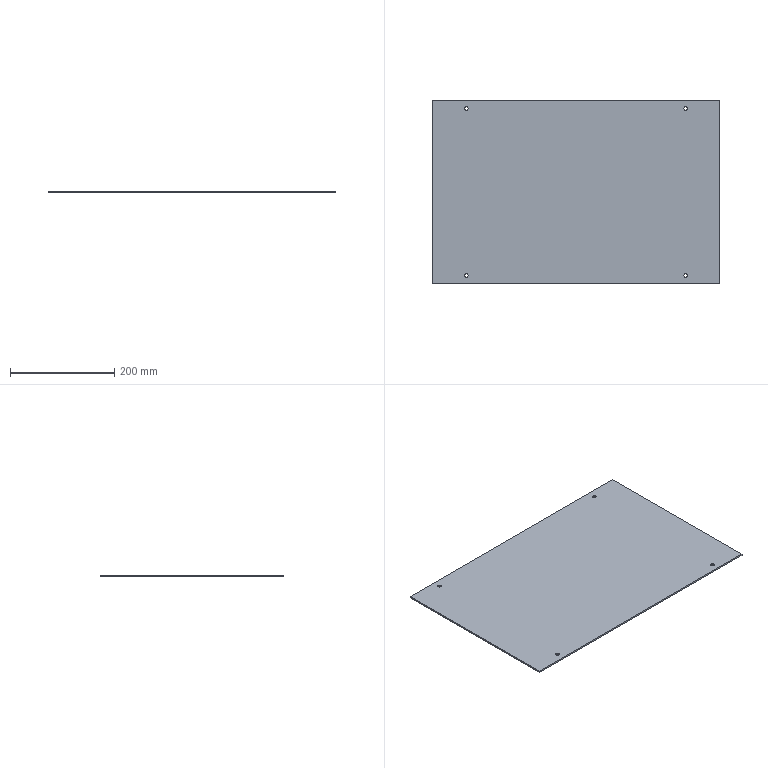Part | SolidWorks | features BaseBody 1 | 1 solid | 14 faces | box 550 x 350 x 3 mm | volume 577089 mm3 | cylinder 8 | plane 6 | commonest cylinder face diameters 6.6 x8
STEP:
#1=CARTESIAN_POINT('',(206.7,160.,0.));
#2=VERTEX_POINT('',#1);
#3=CARTESIAN_POINT('',(213.3,160.,0.));
#4=VERTEX_POINT('',#3);
#5=CARTESIAN_POINT('',(210.,160.,0.));
#6=DIRECTION('',(0.,0.,1.));
#7=DIRECTION('',(-1.,0.,0.));
#8=AXIS2_PLACEMENT_3D('',#5,#6,#7);
#9=CIRCLE('',#8,3.3);
#10=EDGE_CURVE('',#2,#4,#9,.T.);
#11=ORIENTED_EDGE('',*,*,#10,.T.);
#12=CARTESIAN_POINT('',(213.3,160.,-3.));
#13=VERTEX_POINT('',#12);
#14=CARTESIAN_POINT('',(213.3,160.,0.));
#15=DIRECTION('',(0.,0.,-1.));
#16=VECTOR('',#15,1000.);
#17=LINE('',#14,#16);
#18=EDGE_CURVE('',#4,#13,#17,.T.);
#19=ORIENTED_EDGE('',*,*,#18,.T.);
#20=CARTESIAN_POINT('',(206.7,160.,-3.));
#21=VERTEX_POINT('',#20);
#22=CARTESIAN_POINT('',(210.,160.,-3.));
#23=DIRECTION('',(0.,0.,-1.));
#24=DIRECTION('',(-1.,0.,0.));
#25=AXIS2_PLACEMENT_3D('',#22,#23,#24);
#26=CIRCLE('',#25,3.3);
#27=EDGE_CURVE('',#13,#21,#26,.T.);
#28=ORIENTED_EDGE('',*,*,#27,.T.);
#29=CARTESIAN_POINT('',(206.7,160.,0.));
#30=DIRECTION('',(0.,0.,-1.));
#31=VECTOR('',#30,1000.);
#32=LINE('',#29,#31);
#33=EDGE_CURVE('',#2,#21,#32,.T.);
#34=ORIENTED_EDGE('',*,*,#33,.F.);
#35=EDGE_LOOP('',(#11,#19,#28,#34));
#36=FACE_OUTER_BOUND('',#35,.T.);
#37=CARTESIAN_POINT('',(210.,160.,0.));
#38=DIRECTION('',(0.,0.,-1.));
#39=DIRECTION('',(-1.,0.,0.));
#40=AXIS2_PLACEMENT_3D('',#37,#38,#39);
#41=CYLINDRICAL_SURFACE('',#40,3.3);
#42=ADVANCED_FACE('',(#36),#41,.F.);
#43=CARTESIAN_POINT('',(-213.3,160.,0.));
#44=VERTEX_POINT('',#43);
#45=CARTESIAN_POINT('',(-206.7,160.,0.));
#46=VERTEX_POINT('',#45);
#47=CARTESIAN_POINT('',(-210.,160.,0.));
#48=DIRECTION('',(0.,0.,1.));
#49=DIRECTION('',(-1.,0.,0.));
#50=AXIS2_PLACEMENT_3D('',#47,#48,#49);
#51=CIRCLE('',#50,3.3);
#52=EDGE_CURVE('',#44,#46,#51,.T.);
#53=ORIENTED_EDGE('',*,*,#52,.T.);
#54=CARTESIAN_POINT('',(-206.7,160.,-3.));
#55=VERTEX_POINT('',#54);
#56=CARTESIAN_POINT('',(-206.7,160.,0.));
#57=DIRECTION('',(0.,0.,-1.));
#58=VECTOR('',#57,1000.);
#59=LINE('',#56,#58);
#60=EDGE_CURVE('',#46,#55,#59,.T.);
#61=ORIENTED_EDGE('',*,*,#60,.T.);
#62=CARTESIAN_POINT('',(-213.3,160.,-3.));
#63=VERTEX_POINT('',#62);
#64=CARTESIAN_POINT('',(-210.,160.,-3.));
#65=DIRECTION('',(0.,0.,1.));
#66=DIRECTION('',(-1.,0.,0.));
#67=AXIS2_PLACEMENT_3D('',#64,#65,#66);
#68=CIRCLE('',#67,3.3);
#69=EDGE_CURVE('',#63,#55,#68,.T.);
#70=ORIENTED_EDGE('',*,*,#69,.F.);
#71=CARTESIAN_POINT('',(-213.3,160.,0.));
#72=DIRECTION('',(0.,0.,-1.));
#73=VECTOR('',#72,1000.);
#74=LINE('',#71,#73);
#75=EDGE_CURVE('',#44,#63,#74,.T.);
#76=ORIENTED_EDGE('',*,*,#75,.F.);
#77=EDGE_LOOP('',(#53,#61,#70,#76));
#78=FACE_OUTER_BOUND('',#77,.T.);
#79=CARTESIAN_POINT('',(-210.,160.,0.));
#80=DIRECTION('',(0.,0.,-1.));
#81=DIRECTION('',(-1.,0.,0.));
#82=AXIS2_PLACEMENT_3D('',#79,#80,#81);
#83=CYLINDRICAL_SURFACE('',#82,3.3);
#84=ADVANCED_FACE('',(#78),#83,.F.);
#85=CARTESIAN_POINT('',(-213.3,-160.,0.));
#86=VERTEX_POINT('',#85);
#87=CARTESIAN_POINT('',(-206.7,-160.,0.));
#88=VERTEX_POINT('',#87);
#89=CARTESIAN_POINT('',(-210.,-160.,0.));
#90=DIRECTION('',(0.,0.,1.));
#91=DIRECTION('',(-1.,0.,0.));
#92=AXIS2_PLACEMENT_3D('',#89,#90,#91);
#93=CIRCLE('',#92,3.3);
#94=EDGE_CURVE('',#86,#88,#93,.T.);
#95=ORIENTED_EDGE('',*,*,#94,.T.);
#96=CARTESIAN_POINT('',(-206.7,-160.,-3.));
#97=VERTEX_POINT('',#96);
#98=CARTESIAN_POINT('',(-206.7,-160.,0.));
#99=DIRECTION('',(0.,0.,-1.));
#100=VECTOR('',#99,1000.);
#101=LINE('',#98,#100);
#102=EDGE_CURVE('',#88,#97,#101,.T.);
#103=ORIENTED_EDGE('',*,*,#102,.T.);
#104=CARTESIAN_POINT('',(-213.3,-160.,-3.));
#105=VERTEX_POINT('',#104);
#106=CARTESIAN_POINT('',(-210.,-160.,-3.));
#107=DIRECTION('',(0.,0.,1.));
#108=DIRECTION('',(-1.,0.,0.));
#109=AXIS2_PLACEMENT_3D('',#106,#107,#108);
#110=CIRCLE('',#109,3.3);
#111=EDGE_CURVE('',#105,#97,#110,.T.);
#112=ORIENTED_EDGE('',*,*,#111,.F.);
#113=CARTESIAN_POINT('',(-213.3,-160.,0.));
#114=DIRECTION('',(0.,0.,-1.));
#115=VECTOR('',#114,1000.);
#116=LINE('',#113,#115);
#117=EDGE_CURVE('',#86,#105,#116,.T.);
#118=ORIENTED_EDGE('',*,*,#117,.F.);
#119=EDGE_LOOP('',(#95,#103,#112,#118));
#120=FACE_OUTER_BOUND('',#119,.T.);
#121=CARTESIAN_POINT('',(-210.,-160.,0.));
#122=DIRECTION('',(0.,0.,-1.));
#123=DIRECTION('',(-1.,0.,0.));
#124=AXIS2_PLACEMENT_3D('',#121,#122,#123);
#125=CYLINDRICAL_SURFACE('',#124,3.3);
#126=ADVANCED_FACE('',(#120),#125,.F.);
#127=CARTESIAN_POINT('',(206.7,-160.,0.));
#128=VERTEX_POINT('',#127);
#129=CARTESIAN_POINT('',(213.3,-160.,0.));
#130=VERTEX_POINT('',#129);
#131=CARTESIAN_POINT('',(210.,-160.,0.));
#132=DIRECTION('',(0.,0.,1.));
#133=DIRECTION('',(-1.,0.,0.));
#134=AXIS2_PLACEMENT_3D('',#131,#132,#133);
#135=CIRCLE('',#134,3.3);
#136=EDGE_CURVE('',#128,#130,#135,.T.);
#137=ORIENTED_EDGE('',*,*,#136,.T.);
#138=CARTESIAN_POINT('',(213.3,-160.,-3.));
#139=VERTEX_POINT('',#138);
#140=CARTESIAN_POINT('',(213.3,-160.,0.));
#141=DIRECTION('',(0.,0.,-1.));
#142=VECTOR('',#141,1000.);
#143=LINE('',#140,#142);
#144=EDGE_CURVE('',#130,#139,#143,.T.);
#145=ORIENTED_EDGE('',*,*,#144,.T.);
#146=CARTESIAN_POINT('',(206.7,-160.,-3.));
#147=VERTEX_POINT('',#146);
#148=CARTESIAN_POINT('',(210.,-160.,-3.));
#149=DIRECTION('',(0.,0.,1.));
#150=DIRECTION('',(-1.,0.,0.));
#151=AXIS2_PLACEMENT_3D('',#148,#149,#150);
#152=CIRCLE('',#151,3.3);
#153=EDGE_CURVE('',#147,#139,#152,.T.);
#154=ORIENTED_EDGE('',*,*,#153,.F.);
#155=CARTESIAN_POINT('',(206.7,-160.,0.));
#156=DIRECTION('',(0.,0.,-1.));
#157=VECTOR('',#156,1000.);
#158=LINE('',#155,#157);
#159=EDGE_CURVE('',#128,#147,#158,.T.);
#160=ORIENTED_EDGE('',*,*,#159,.F.);
#161=EDGE_LOOP('',(#137,#145,#154,#160));
#162=FACE_OUTER_BOUND('',#161,.T.);
#163=CARTESIAN_POINT('',(210.,-160.,0.));
#164=DIRECTION('',(0.,0.,-1.));
#165=DIRECTION('',(-1.,0.,0.));
#166=AXIS2_PLACEMENT_3D('',#163,#164,#165);
#167=CYLINDRICAL_SURFACE('',#166,3.3);
#168=ADVANCED_FACE('',(#162),#167,.F.);
#169=ORIENTED_EDGE('',*,*,#18,.F.);
#170=CARTESIAN_POINT('',(210.,160.,0.));
#171=DIRECTION('',(0.,0.,1.));
#172=DIRECTION('',(-1.,0.,0.));
#173=AXIS2_PLACEMENT_3D('',#170,#171,#172);
#174=CIRCLE('',#173,3.3);
#175=EDGE_CURVE('',#4,#2,#174,.T.);
#176=ORIENTED_EDGE('',*,*,#175,.T.);
#177=ORIENTED_EDGE('',*,*,#33,.T.);
#178=CARTESIAN_POINT('',(210.,160.,-3.));
#179=DIRECTION('',(0.,0.,-1.));
#180=DIRECTION('',(-1.,0.,0.));
#181=AXIS2_PLACEMENT_3D('',#178,#179,#180);
#182=CIRCLE('',#181,3.3);
#183=EDGE_CURVE('',#21,#13,#182,.T.);
#184=ORIENTED_EDGE('',*,*,#183,.T.);
#185=EDGE_LOOP('',(#169,#176,#177,#184));
#186=FACE_OUTER_BOUND('',#185,.T.);
#187=CARTESIAN_POINT('',(210.,160.,0.));
#188=DIRECTION('',(0.,0.,-1.));
#189=DIRECTION('',(-1.,0.,0.));
#190=AXIS2_PLACEMENT_3D('',#187,#188,#189);
#191=CYLINDRICAL_SURFACE('',#190,3.3);
#192=ADVANCED_FACE('',(#186),#191,.F.);
#193=ORIENTED_EDGE('',*,*,#69,.T.);
#194=CARTESIAN_POINT('',(-210.,160.,-3.));
#195=DIRECTION('',(0.,0.,1.));
#196=DIRECTION('',(-1.,0.,0.));
#197=AXIS2_PLACEMENT_3D('',#194,#195,#196);
#198=CIRCLE('',#197,3.3);
#199=EDGE_CURVE('',#55,#63,#198,.T.);
#200=ORIENTED_EDGE('',*,*,#199,.T.);
#201=EDGE_LOOP('',(#193,#200));
#202=FACE_BOUND('',#201,.T.);
#203=ORIENTED_EDGE('',*,*,#111,.T.);
#204=CARTESIAN_POINT('',(-210.,-160.,-3.));
#205=DIRECTION('',(0.,0.,1.));
#206=DIRECTION('',(-1.,0.,0.));
#207=AXIS2_PLACEMENT_3D('',#204,#205,#206);
#208=CIRCLE('',#207,3.3);
#209=EDGE_CURVE('',#97,#105,#208,.T.);
#210=ORIENTED_EDGE('',*,*,#209,.T.);
#211=EDGE_LOOP('',(#203,#210));
#212=FACE_BOUND('',#211,.T.);
#213=ORIENTED_EDGE('',*,*,#153,.T.);
#214=CARTESIAN_POINT('',(210.,-160.,-3.));
#215=DIRECTION('',(0.,0.,1.));
#216=DIRECTION('',(-1.,0.,0.));
#217=AXIS2_PLACEMENT_3D('',#214,#215,#216);
#218=CIRCLE('',#217,3.3);
#219=EDGE_CURVE('',#139,#147,#218,.T.);
#220=ORIENTED_EDGE('',*,*,#219,.T.);
#221=EDGE_LOOP('',(#213,#220));
#222=FACE_BOUND('',#221,.T.);
#223=ORIENTED_EDGE('',*,*,#183,.F.);
#224=ORIENTED_EDGE('',*,*,#27,.F.);
#225=EDGE_LOOP('',(#223,#224));
#226=FACE_BOUND('',#225,.T.);
#227=CARTESIAN_POINT('',(-275.,-175.,-3.));
#228=VERTEX_POINT('',#227);
#229=CARTESIAN_POINT('',(-275.,175.,-3.));
#230=VERTEX_POINT('',#229);
#231=CARTESIAN_POINT('',(-275.,0.,-3.));
#232=DIRECTION('',(0.,1.,0.));
#233=VECTOR('',#232,1000.);
#234=LINE('',#231,#233);
#235=EDGE_CURVE('',#228,#230,#234,.T.);
#236=ORIENTED_EDGE('',*,*,#235,.T.);
#237=CARTESIAN_POINT('',(275.,175.,-3.));
#238=VERTEX_POINT('',#237);
#239=CARTESIAN_POINT('',(0.,175.,-3.));
#240=DIRECTION('',(1.,0.,0.));
#241=VECTOR('',#240,1000.);
#242=LINE('',#239,#241);
#243=EDGE_CURVE('',#230,#238,#242,.T.);
#244=ORIENTED_EDGE('',*,*,#243,.T.);
#245=CARTESIAN_POINT('',(275.,-175.,-3.));
#246=VERTEX_POINT('',#245);
#247=CARTESIAN_POINT('',(275.,0.,-3.));
#248=DIRECTION('',(0.,-1.,0.));
#249=VECTOR('',#248,1000.);
#250=LINE('',#247,#249);
#251=EDGE_CURVE('',#238,#246,#250,.T.);
#252=ORIENTED_EDGE('',*,*,#251,.T.);
#253=CARTESIAN_POINT('',(0.,-175.,-3.));
#254=DIRECTION('',(-1.,0.,0.));
#255=VECTOR('',#254,1000.);
#256=LINE('',#253,#255);
#257=EDGE_CURVE('',#246,#228,#256,.T.);
#258=ORIENTED_EDGE('',*,*,#257,.T.);
#259=EDGE_LOOP('',(#236,#244,#252,#258));
#260=FACE_OUTER_BOUND('',#259,.T.);
#261=CARTESIAN_POINT('',(275.,-175.,-3.));
#262=DIRECTION('',(0.,0.,-1.));
#263=DIRECTION('',(-1.,0.,0.));
#264=AXIS2_PLACEMENT_3D('',#261,#262,#263);
#265=PLANE('',#264);
#266=ADVANCED_FACE('',(#202,#212,#222,#226,#260),#265,.T.);
#267=ORIENTED_EDGE('',*,*,#52,.F.);
#268=CARTESIAN_POINT('',(-210.,160.,0.));
#269=DIRECTION('',(0.,0.,1.));
#270=DIRECTION('',(-1.,0.,0.));
#271=AXIS2_PLACEMENT_3D('',#268,#269,#270);
#272=CIRCLE('',#271,3.3);
#273=EDGE_CURVE('',#46,#44,#272,.T.);
#274=ORIENTED_EDGE('',*,*,#273,.F.);
#275=EDGE_LOOP('',(#267,#274));
#276=FACE_BOUND('',#275,.T.);
#277=ORIENTED_EDGE('',*,*,#94,.F.);
#278=CARTESIAN_POINT('',(-210.,-160.,0.));
#279=DIRECTION('',(0.,0.,1.));
#280=DIRECTION('',(-1.,0.,0.));
#281=AXIS2_PLACEMENT_3D('',#278,#279,#280);
#282=CIRCLE('',#281,3.3);
#283=EDGE_CURVE('',#88,#86,#282,.T.);
#284=ORIENTED_EDGE('',*,*,#283,.F.);
#285=EDGE_LOOP('',(#277,#284));
#286=FACE_BOUND('',#285,.T.);
#287=ORIENTED_EDGE('',*,*,#136,.F.);
#288=CARTESIAN_POINT('',(210.,-160.,0.));
#289=DIRECTION('',(0.,0.,1.));
#290=DIRECTION('',(-1.,0.,0.));
#291=AXIS2_PLACEMENT_3D('',#288,#289,#290);
#292=CIRCLE('',#291,3.3);
#293=EDGE_CURVE('',#130,#128,#292,.T.);
#294=ORIENTED_EDGE('',*,*,#293,.F.);
#295=EDGE_LOOP('',(#287,#294));
#296=FACE_BOUND('',#295,.T.);
#297=ORIENTED_EDGE('',*,*,#10,.F.);
#298=ORIENTED_EDGE('',*,*,#175,.F.);
#299=EDGE_LOOP('',(#297,#298));
#300=FACE_BOUND('',#299,.T.);
#301=CARTESIAN_POINT('',(-275.,175.,0.));
#302=VERTEX_POINT('',#301);
#303=CARTESIAN_POINT('',(275.,175.,0.));
#304=VERTEX_POINT('',#303);
#305=CARTESIAN_POINT('',(0.,175.,0.));
#306=DIRECTION('',(1.,0.,0.));
#307=VECTOR('',#306,1000.);
#308=LINE('',#305,#307);
#309=EDGE_CURVE('',#302,#304,#308,.T.);
#310=ORIENTED_EDGE('',*,*,#309,.F.);
#311=CARTESIAN_POINT('',(-275.,-175.,0.));
#312=VERTEX_POINT('',#311);
#313=CARTESIAN_POINT('',(-275.,0.,0.));
#314=DIRECTION('',(0.,1.,0.));
#315=VECTOR('',#314,1000.);
#316=LINE('',#313,#315);
#317=EDGE_CURVE('',#312,#302,#316,.T.);
#318=ORIENTED_EDGE('',*,*,#317,.F.);
#319=CARTESIAN_POINT('',(275.,-175.,0.));
#320=VERTEX_POINT('',#319);
#321=CARTESIAN_POINT('',(0.,-175.,0.));
#322=DIRECTION('',(-1.,0.,0.));
#323=VECTOR('',#322,1000.);
#324=LINE('',#321,#323);
#325=EDGE_CURVE('',#320,#312,#324,.T.);
#326=ORIENTED_EDGE('',*,*,#325,.F.);
#327=CARTESIAN_POINT('',(275.,0.,0.));
#328=DIRECTION('',(0.,-1.,0.));
#329=VECTOR('',#328,1000.);
#330=LINE('',#327,#329);
#331=EDGE_CURVE('',#304,#320,#330,.T.);
#332=ORIENTED_EDGE('',*,*,#331,.F.);
#333=EDGE_LOOP('',(#310,#318,#326,#332));
#334=FACE_OUTER_BOUND('',#333,.T.);
#335=CARTESIAN_POINT('',(275.,-175.,0.));
#336=DIRECTION('',(0.,0.,-1.));
#337=DIRECTION('',(-1.,0.,0.));
#338=AXIS2_PLACEMENT_3D('',#335,#336,#337);
#339=PLANE('',#338);
#340=ADVANCED_FACE('',(#276,#286,#296,#300,#334),#339,.F.);
#341=ORIENTED_EDGE('',*,*,#60,.F.);
#342=ORIENTED_EDGE('',*,*,#273,.T.);
#343=ORIENTED_EDGE('',*,*,#75,.T.);
#344=ORIENTED_EDGE('',*,*,#199,.F.);
#345=EDGE_LOOP('',(#341,#342,#343,#344));
#346=FACE_OUTER_BOUND('',#345,.T.);
#347=CARTESIAN_POINT('',(-210.,160.,0.));
#348=DIRECTION('',(0.,0.,-1.));
#349=DIRECTION('',(-1.,0.,0.));
#350=AXIS2_PLACEMENT_3D('',#347,#348,#349);
#351=CYLINDRICAL_SURFACE('',#350,3.3);
#352=ADVANCED_FACE('',(#346),#351,.F.);
#353=ORIENTED_EDGE('',*,*,#102,.F.);
#354=ORIENTED_EDGE('',*,*,#283,.T.);
#355=ORIENTED_EDGE('',*,*,#117,.T.);
#356=ORIENTED_EDGE('',*,*,#209,.F.);
#357=EDGE_LOOP('',(#353,#354,#355,#356));
#358=FACE_OUTER_BOUND('',#357,.T.);
#359=CARTESIAN_POINT('',(-210.,-160.,0.));
#360=DIRECTION('',(0.,0.,-1.));
#361=DIRECTION('',(-1.,0.,0.));
#362=AXIS2_PLACEMENT_3D('',#359,#360,#361);
#363=CYLINDRICAL_SURFACE('',#362,3.3);
#364=ADVANCED_FACE('',(#358),#363,.F.);
#365=ORIENTED_EDGE('',*,*,#144,.F.);
#366=ORIENTED_EDGE('',*,*,#293,.T.);
#367=ORIENTED_EDGE('',*,*,#159,.T.);
#368=ORIENTED_EDGE('',*,*,#219,.F.);
#369=EDGE_LOOP('',(#365,#366,#367,#368));
#370=FACE_OUTER_BOUND('',#369,.T.);
#371=CARTESIAN_POINT('',(210.,-160.,0.));
#372=DIRECTION('',(0.,0.,-1.));
#373=DIRECTION('',(-1.,0.,0.));
#374=AXIS2_PLACEMENT_3D('',#371,#372,#373);
#375=CYLINDRICAL_SURFACE('',#374,3.3);
#376=ADVANCED_FACE('',(#370),#375,.F.);
#377=ORIENTED_EDGE('',*,*,#243,.F.);
#378=CARTESIAN_POINT('',(-275.,175.,-1.5));
#379=DIRECTION('',(0.,0.,1.));
#380=VECTOR('',#379,1000.);
#381=LINE('',#378,#380);
#382=EDGE_CURVE('',#230,#302,#381,.T.);
#383=ORIENTED_EDGE('',*,*,#382,.T.);
#384=ORIENTED_EDGE('',*,*,#309,.T.);
#385=CARTESIAN_POINT('',(275.,175.,-1.5));
#386=DIRECTION('',(0.,0.,-1.));
#387=VECTOR('',#386,1000.);
#388=LINE('',#385,#387);
#389=EDGE_CURVE('',#304,#238,#388,.T.);
#390=ORIENTED_EDGE('',*,*,#389,.T.);
#391=EDGE_LOOP('',(#377,#383,#384,#390));
#392=FACE_OUTER_BOUND('',#391,.T.);
#393=CARTESIAN_POINT('',(-275.,175.,-3.));
#394=DIRECTION('',(0.,1.,0.));
#395=DIRECTION('',(0.,0.,1.));
#396=AXIS2_PLACEMENT_3D('',#393,#394,#395);
#397=PLANE('',#396);
#398=ADVANCED_FACE('',(#392),#397,.T.);
#399=ORIENTED_EDGE('',*,*,#235,.F.);
#400=CARTESIAN_POINT('',(-275.,-175.,-1.5));
#401=DIRECTION('',(0.,0.,1.));
#402=VECTOR('',#401,1000.);
#403=LINE('',#400,#402);
#404=EDGE_CURVE('',#228,#312,#403,.T.);
#405=ORIENTED_EDGE('',*,*,#404,.T.);
#406=ORIENTED_EDGE('',*,*,#317,.T.);
#407=ORIENTED_EDGE('',*,*,#382,.F.);
#408=EDGE_LOOP('',(#399,#405,#406,#407));
#409=FACE_OUTER_BOUND('',#408,.T.);
#410=CARTESIAN_POINT('',(-275.,-175.,-3.));
#411=DIRECTION('',(-1.,0.,0.));
#412=DIRECTION('',(0.,0.,1.));
#413=AXIS2_PLACEMENT_3D('',#410,#411,#412);
#414=PLANE('',#413);
#415=ADVANCED_FACE('',(#409),#414,.T.);
#416=ORIENTED_EDGE('',*,*,#257,.F.);
#417=CARTESIAN_POINT('',(275.,-175.,-1.5));
#418=DIRECTION('',(0.,0.,1.));
#419=VECTOR('',#418,1000.);
#420=LINE('',#417,#419);
#421=EDGE_CURVE('',#246,#320,#420,.T.);
#422=ORIENTED_EDGE('',*,*,#421,.T.);
#423=ORIENTED_EDGE('',*,*,#325,.T.);
#424=ORIENTED_EDGE('',*,*,#404,.F.);
#425=EDGE_LOOP('',(#416,#422,#423,#424));
#426=FACE_OUTER_BOUND('',#425,.T.);
#427=CARTESIAN_POINT('',(-275.,-175.,0.));
#428=DIRECTION('',(0.,-1.,0.));
#429=DIRECTION('',(0.,0.,-1.));
#430=AXIS2_PLACEMENT_3D('',#427,#428,#429);
#431=PLANE('',#430);
#432=ADVANCED_FACE('',(#426),#431,.T.);
#433=ORIENTED_EDGE('',*,*,#251,.F.);
#434=ORIENTED_EDGE('',*,*,#389,.F.);
#435=ORIENTED_EDGE('',*,*,#331,.T.);
#436=ORIENTED_EDGE('',*,*,#421,.F.);
#437=EDGE_LOOP('',(#433,#434,#435,#436));
#438=FACE_OUTER_BOUND('',#437,.T.);
#439=CARTESIAN_POINT('',(275.,-175.,0.));
#440=DIRECTION('',(1.,0.,0.));
#441=DIRECTION('',(0.,0.,-1.));
#442=AXIS2_PLACEMENT_3D('',#439,#440,#441);
#443=PLANE('',#442);
#444=ADVANCED_FACE('',(#438),#443,.T.);
#445=CLOSED_SHELL('',(#42,#84,#126,#168,#192,#266,#340,#352,#364,#376,#398,#415,#432,#444));
#446=MANIFOLD_SOLID_BREP('',#445);
#447=CARTESIAN_POINT('',(0.,0.,0.));
#448=DIRECTION('',(0.,0.,1.));
#449=DIRECTION('',(1.,0.,0.));
#450=AXIS2_PLACEMENT_3D('',#447,#448,#449);
#451=(LENGTH_UNIT()NAMED_UNIT(*)SI_UNIT(.MILLI.,.METRE.));
#452=UNCERTAINTY_MEASURE_WITH_UNIT(LENGTH_MEASURE(0.00001),#451,'','');
#453=(NAMED_UNIT(*)PLANE_ANGLE_UNIT()SI_UNIT($,.RADIAN.));
#454=(NAMED_UNIT(*)SI_UNIT($,.STERADIAN.)SOLID_ANGLE_UNIT());
#455=(GEOMETRIC_REPRESENTATION_CONTEXT(3)GLOBAL_UNCERTAINTY_ASSIGNED_CONTEXT((#452))GLOBAL_UNIT_ASSIGNED_CONTEXT((#451,#453,#454))REPRESENTATION_CONTEXT('',''));
#456=ADVANCED_BREP_SHAPE_REPRESENTATION('',(#446,#450),#455);